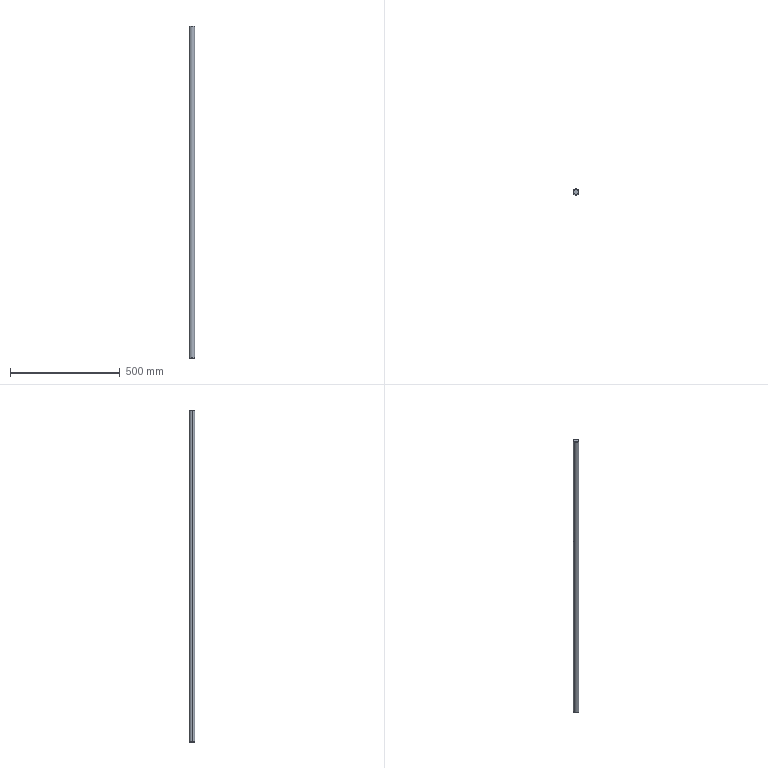Part | STEP file | 1 solid | 8 faces | box 25 x 25 x 1510 mm | volume 741143 mm3 | cone 4 | cylinder 2 | plane 2 | commonest cylinder face diameters 25 x2
STEP:
#1=CARTESIAN_POINT('',(0.,0.,0.));
#2=DIRECTION('',(0.,0.,1.));
#3=DIRECTION('',(1.,0.,0.));
#4=AXIS2_PLACEMENT_3D('',#1,#2,#3);
#5=CARTESIAN_POINT('',(-11.5,0.,-755.));
#6=VERTEX_POINT('',#5);
#7=CARTESIAN_POINT('',(11.5,0.,-755.));
#8=VERTEX_POINT('',#7);
#9=CARTESIAN_POINT('',(0.,0.,-755.));
#10=DIRECTION('',(0.,0.,-1.));
#11=DIRECTION('',(1.,0.,0.));
#12=AXIS2_PLACEMENT_3D('',#9,#10,#11);
#13=CIRCLE('',#12,11.5);
#14=CARTESIAN_POINT('',(0.,0.,-754.));
#15=DIRECTION('',(0.,0.,1.));
#16=DIRECTION('',(1.,0.,0.));
#17=AXIS2_PLACEMENT_3D('',#14,#15,#16);
#18=CONICAL_SURFACE('',#17,12.5,0.7854);
#19=CARTESIAN_POINT('',(6.283,-1.));
#20=DIRECTION('',(-1.,0.));
#21=VECTOR('',#20,1.);
#22=LINE('',#19,#21);
#23=(GEOMETRIC_REPRESENTATION_CONTEXT(2)PARAMETRIC_REPRESENTATION_CONTEXT()REPRESENTATION_CONTEXT('',''));
#24=DEFINITIONAL_REPRESENTATION('',(#22),#23);
#25=PCURVE('',#18,#24);
#26=CARTESIAN_POINT('',(0.,0.,-755.));
#27=DIRECTION('',(0.,0.,1.));
#28=DIRECTION('',(1.,0.,0.));
#29=AXIS2_PLACEMENT_3D('',#26,#27,#28);
#30=PLANE('',#29);
#31=CARTESIAN_POINT('',(11.5,0.));
#32=CARTESIAN_POINT('',(11.5,-19.919));
#33=CARTESIAN_POINT('',(-5.75,-9.959));
#34=CARTESIAN_POINT('',(-23.,0.));
#35=CARTESIAN_POINT('',(-5.75,9.959));
#36=CARTESIAN_POINT('',(11.5,19.919));
#37=CARTESIAN_POINT('',(11.5,0.));
#38=(BOUNDED_CURVE()B_SPLINE_CURVE(2,(#31,#32,#33,#34,#35,#36,#37),.UNSPECIFIED.,.T.,.F.)B_SPLINE_CURVE_WITH_KNOTS((1,2,2,2,2,1),(-2.094,0.,2.094,4.189,6.283,8.378),.UNSPECIFIED.)CURVE()GEOMETRIC_REPRESENTATION_ITEM()RATIONAL_B_SPLINE_CURVE((1.,0.5,1.,0.5,1.,0.5,1.))REPRESENTATION_ITEM(''));
#39=(GEOMETRIC_REPRESENTATION_CONTEXT(2)PARAMETRIC_REPRESENTATION_CONTEXT()REPRESENTATION_CONTEXT('',''));
#40=DEFINITIONAL_REPRESENTATION('',(#38),#39);
#41=PCURVE('',#30,#40);
#42=SURFACE_CURVE('',#13,(#25,#41),.PCURVE_S1.);
#43=EDGE_CURVE('',#6,#8,#42,.T.);
#44=ORIENTED_EDGE('',*,*,#43,.F.);
#45=CARTESIAN_POINT('',(-12.5,0.,-754.));
#46=VERTEX_POINT('',#45);
#47=CARTESIAN_POINT('',(-12.5,0.,-754.));
#48=DIRECTION('',(-0.7071,0.,0.7071));
#49=VECTOR('',#48,1.);
#50=LINE('',#47,#49);
#51=CARTESIAN_POINT('',(3.142,0.));
#52=DIRECTION('',(0.,1.));
#53=VECTOR('',#52,1.);
#54=LINE('',#51,#53);
#55=(GEOMETRIC_REPRESENTATION_CONTEXT(2)PARAMETRIC_REPRESENTATION_CONTEXT()REPRESENTATION_CONTEXT('',''));
#56=DEFINITIONAL_REPRESENTATION('',(#54),#55);
#57=PCURVE('',#18,#56);
#58=CARTESIAN_POINT('',(0.,0.,-754.));
#59=DIRECTION('',(0.,0.,1.));
#60=DIRECTION('',(1.,0.,0.));
#61=AXIS2_PLACEMENT_3D('',#58,#59,#60);
#62=CONICAL_SURFACE('',#61,12.5,0.7854);
#63=CARTESIAN_POINT('',(3.142,0.));
#64=DIRECTION('',(0.,1.));
#65=VECTOR('',#64,1.);
#66=LINE('',#63,#65);
#67=(GEOMETRIC_REPRESENTATION_CONTEXT(2)PARAMETRIC_REPRESENTATION_CONTEXT()REPRESENTATION_CONTEXT('',''));
#68=DEFINITIONAL_REPRESENTATION('',(#66),#67);
#69=PCURVE('',#62,#68);
#70=SURFACE_CURVE('',#50,(#57,#69),.PCURVE_S1.);
#71=EDGE_CURVE('',#6,#46,#70,.T.);
#72=ORIENTED_EDGE('',*,*,#71,.T.);
#73=CARTESIAN_POINT('',(12.5,0.,-754.));
#74=VERTEX_POINT('',#73);
#75=CARTESIAN_POINT('',(0.,0.,-754.));
#76=DIRECTION('',(0.,0.,1.));
#77=DIRECTION('',(1.,0.,0.));
#78=AXIS2_PLACEMENT_3D('',#75,#76,#77);
#79=CIRCLE('',#78,12.5);
#80=CARTESIAN_POINT('',(0.,0.));
#81=DIRECTION('',(1.,0.));
#82=VECTOR('',#81,1.);
#83=LINE('',#80,#82);
#84=(GEOMETRIC_REPRESENTATION_CONTEXT(2)PARAMETRIC_REPRESENTATION_CONTEXT()REPRESENTATION_CONTEXT('',''));
#85=DEFINITIONAL_REPRESENTATION('',(#83),#84);
#86=PCURVE('',#18,#85);
#87=CARTESIAN_POINT('',(0.,0.,755.));
#88=DIRECTION('',(0.,0.,-1.));
#89=DIRECTION('',(-1.,0.,0.));
#90=AXIS2_PLACEMENT_3D('',#87,#88,#89);
#91=CYLINDRICAL_SURFACE('',#90,12.5);
#92=CARTESIAN_POINT('',(3.142,1509.));
#93=DIRECTION('',(-1.,0.));
#94=VECTOR('',#93,1.);
#95=LINE('',#92,#94);
#96=(GEOMETRIC_REPRESENTATION_CONTEXT(2)PARAMETRIC_REPRESENTATION_CONTEXT()REPRESENTATION_CONTEXT('',''));
#97=DEFINITIONAL_REPRESENTATION('',(#95),#96);
#98=PCURVE('',#91,#97);
#99=SURFACE_CURVE('',#79,(#86,#98),.PCURVE_S1.);
#100=EDGE_CURVE('',#74,#46,#99,.T.);
#101=ORIENTED_EDGE('',*,*,#100,.F.);
#102=CARTESIAN_POINT('',(12.5,0.,-754.));
#103=DIRECTION('',(0.7071,0.,0.7071));
#104=VECTOR('',#103,1.);
#105=LINE('',#102,#104);
#106=CARTESIAN_POINT('',(0.,0.));
#107=DIRECTION('',(0.,1.));
#108=VECTOR('',#107,1.);
#109=LINE('',#106,#108);
#110=(GEOMETRIC_REPRESENTATION_CONTEXT(2)PARAMETRIC_REPRESENTATION_CONTEXT()REPRESENTATION_CONTEXT('',''));
#111=DEFINITIONAL_REPRESENTATION('',(#109),#110);
#112=PCURVE('',#18,#111);
#113=CARTESIAN_POINT('',(6.283,0.));
#114=DIRECTION('',(0.,1.));
#115=VECTOR('',#114,1.);
#116=LINE('',#113,#115);
#117=(GEOMETRIC_REPRESENTATION_CONTEXT(2)PARAMETRIC_REPRESENTATION_CONTEXT()REPRESENTATION_CONTEXT('',''));
#118=DEFINITIONAL_REPRESENTATION('',(#116),#117);
#119=PCURVE('',#62,#118);
#120=SURFACE_CURVE('',#105,(#112,#119),.PCURVE_S1.);
#121=EDGE_CURVE('',#8,#74,#120,.T.);
#122=ORIENTED_EDGE('',*,*,#121,.F.);
#123=EDGE_LOOP('',(#44,#72,#101,#122));
#124=FACE_BOUND('',#123,.T.);
#125=ADVANCED_FACE('',(#124),#18,.T.);
#126=CARTESIAN_POINT('',(11.5,0.,755.));
#127=VERTEX_POINT('',#126);
#128=CARTESIAN_POINT('',(-11.5,0.,755.));
#129=VERTEX_POINT('',#128);
#130=CARTESIAN_POINT('',(0.,0.,755.));
#131=DIRECTION('',(0.,0.,1.));
#132=DIRECTION('',(1.,0.,0.));
#133=AXIS2_PLACEMENT_3D('',#130,#131,#132);
#134=CIRCLE('',#133,11.5);
#135=CARTESIAN_POINT('',(0.,0.,755.));
#136=DIRECTION('',(0.,0.,-1.));
#137=DIRECTION('',(-1.,0.,0.));
#138=AXIS2_PLACEMENT_3D('',#135,#136,#137);
#139=CONICAL_SURFACE('',#138,11.5,0.7854);
#140=CARTESIAN_POINT('',(3.142,0.));
#141=DIRECTION('',(-1.,0.));
#142=VECTOR('',#141,1.);
#143=LINE('',#140,#142);
#144=(GEOMETRIC_REPRESENTATION_CONTEXT(2)PARAMETRIC_REPRESENTATION_CONTEXT()REPRESENTATION_CONTEXT('',''));
#145=DEFINITIONAL_REPRESENTATION('',(#143),#144);
#146=PCURVE('',#139,#145);
#147=CARTESIAN_POINT('',(0.,0.,755.));
#148=DIRECTION('',(0.,0.,1.));
#149=DIRECTION('',(1.,0.,0.));
#150=AXIS2_PLACEMENT_3D('',#147,#148,#149);
#151=PLANE('',#150);
#152=CARTESIAN_POINT('',(0.,0.));
#153=DIRECTION('',(1.,0.));
#154=AXIS2_PLACEMENT_2D('',#152,#153);
#155=CIRCLE('',#154,11.5);
#156=(GEOMETRIC_REPRESENTATION_CONTEXT(2)PARAMETRIC_REPRESENTATION_CONTEXT()REPRESENTATION_CONTEXT('',''));
#157=DEFINITIONAL_REPRESENTATION('',(#155),#156);
#158=PCURVE('',#151,#157);
#159=SURFACE_CURVE('',#134,(#146,#158),.PCURVE_S1.);
#160=EDGE_CURVE('',#127,#129,#159,.T.);
#161=ORIENTED_EDGE('',*,*,#160,.F.);
#162=CARTESIAN_POINT('',(12.5,0.,754.));
#163=VERTEX_POINT('',#162);
#164=CARTESIAN_POINT('',(11.5,0.,755.));
#165=DIRECTION('',(0.7071,0.,-0.7071));
#166=VECTOR('',#165,1.);
#167=LINE('',#164,#166);
#168=CARTESIAN_POINT('',(3.142,0.));
#169=DIRECTION('',(0.,1.));
#170=VECTOR('',#169,1.);
#171=LINE('',#168,#170);
#172=(GEOMETRIC_REPRESENTATION_CONTEXT(2)PARAMETRIC_REPRESENTATION_CONTEXT()REPRESENTATION_CONTEXT('',''));
#173=DEFINITIONAL_REPRESENTATION('',(#171),#172);
#174=PCURVE('',#139,#173);
#175=CARTESIAN_POINT('',(0.,0.,755.));
#176=DIRECTION('',(0.,0.,-1.));
#177=DIRECTION('',(-1.,0.,0.));
#178=AXIS2_PLACEMENT_3D('',#175,#176,#177);
#179=CONICAL_SURFACE('',#178,11.5,0.7854);
#180=CARTESIAN_POINT('',(3.142,0.));
#181=DIRECTION('',(0.,1.));
#182=VECTOR('',#181,1.);
#183=LINE('',#180,#182);
#184=(GEOMETRIC_REPRESENTATION_CONTEXT(2)PARAMETRIC_REPRESENTATION_CONTEXT()REPRESENTATION_CONTEXT('',''));
#185=DEFINITIONAL_REPRESENTATION('',(#183),#184);
#186=PCURVE('',#179,#185);
#187=SURFACE_CURVE('',#167,(#174,#186),.PCURVE_S1.);
#188=EDGE_CURVE('',#127,#163,#187,.T.);
#189=ORIENTED_EDGE('',*,*,#188,.T.);
#190=CARTESIAN_POINT('',(-12.5,0.,754.));
#191=VERTEX_POINT('',#190);
#192=CARTESIAN_POINT('',(0.,0.,754.));
#193=DIRECTION('',(0.,0.,-1.));
#194=DIRECTION('',(1.,0.,0.));
#195=AXIS2_PLACEMENT_3D('',#192,#193,#194);
#196=CIRCLE('',#195,12.5);
#197=CARTESIAN_POINT('',(-3.142,1.));
#198=DIRECTION('',(1.,0.));
#199=VECTOR('',#198,1.);
#200=LINE('',#197,#199);
#201=(GEOMETRIC_REPRESENTATION_CONTEXT(2)PARAMETRIC_REPRESENTATION_CONTEXT()REPRESENTATION_CONTEXT('',''));
#202=DEFINITIONAL_REPRESENTATION('',(#200),#201);
#203=PCURVE('',#139,#202);
#204=CARTESIAN_POINT('',(-3.142,1.));
#205=DIRECTION('',(1.,0.));
#206=VECTOR('',#205,1.);
#207=LINE('',#204,#206);
#208=(GEOMETRIC_REPRESENTATION_CONTEXT(2)PARAMETRIC_REPRESENTATION_CONTEXT()REPRESENTATION_CONTEXT('',''));
#209=DEFINITIONAL_REPRESENTATION('',(#207),#208);
#210=PCURVE('',#91,#209);
#211=SURFACE_CURVE('',#196,(#203,#210),.PCURVE_S1.);
#212=EDGE_CURVE('',#191,#163,#211,.T.);
#213=ORIENTED_EDGE('',*,*,#212,.F.);
#214=CARTESIAN_POINT('',(-11.5,0.,755.));
#215=DIRECTION('',(-0.7071,0.,-0.7071));
#216=VECTOR('',#215,1.);
#217=LINE('',#214,#216);
#218=CARTESIAN_POINT('',(0.,0.));
#219=DIRECTION('',(0.,1.));
#220=VECTOR('',#219,1.);
#221=LINE('',#218,#220);
#222=(GEOMETRIC_REPRESENTATION_CONTEXT(2)PARAMETRIC_REPRESENTATION_CONTEXT()REPRESENTATION_CONTEXT('',''));
#223=DEFINITIONAL_REPRESENTATION('',(#221),#222);
#224=PCURVE('',#139,#223);
#225=CARTESIAN_POINT('',(6.283,0.));
#226=DIRECTION('',(0.,1.));
#227=VECTOR('',#226,1.);
#228=LINE('',#225,#227);
#229=(GEOMETRIC_REPRESENTATION_CONTEXT(2)PARAMETRIC_REPRESENTATION_CONTEXT()REPRESENTATION_CONTEXT('',''));
#230=DEFINITIONAL_REPRESENTATION('',(#228),#229);
#231=PCURVE('',#179,#230);
#232=SURFACE_CURVE('',#217,(#224,#231),.PCURVE_S1.);
#233=EDGE_CURVE('',#129,#191,#232,.T.);
#234=ORIENTED_EDGE('',*,*,#233,.F.);
#235=EDGE_LOOP('',(#161,#189,#213,#234));
#236=FACE_BOUND('',#235,.T.);
#237=ADVANCED_FACE('',(#236),#139,.T.);
#238=ORIENTED_EDGE('',*,*,#212,.T.);
#239=CARTESIAN_POINT('',(12.5,0.,755.));
#240=DIRECTION('',(0.,0.,-1.));
#241=VECTOR('',#240,1.);
#242=LINE('',#239,#241);
#243=CARTESIAN_POINT('',(3.142,0.));
#244=DIRECTION('',(0.,1.));
#245=VECTOR('',#244,1.);
#246=LINE('',#243,#245);
#247=(GEOMETRIC_REPRESENTATION_CONTEXT(2)PARAMETRIC_REPRESENTATION_CONTEXT()REPRESENTATION_CONTEXT('',''));
#248=DEFINITIONAL_REPRESENTATION('',(#246),#247);
#249=PCURVE('',#91,#248);
#250=CARTESIAN_POINT('',(0.,0.,755.));
#251=DIRECTION('',(0.,0.,-1.));
#252=DIRECTION('',(-1.,0.,0.));
#253=AXIS2_PLACEMENT_3D('',#250,#251,#252);
#254=CYLINDRICAL_SURFACE('',#253,12.5);
#255=CARTESIAN_POINT('',(3.142,0.));
#256=DIRECTION('',(0.,1.));
#257=VECTOR('',#256,1.);
#258=LINE('',#255,#257);
#259=(GEOMETRIC_REPRESENTATION_CONTEXT(2)PARAMETRIC_REPRESENTATION_CONTEXT()REPRESENTATION_CONTEXT('',''));
#260=DEFINITIONAL_REPRESENTATION('',(#258),#259);
#261=PCURVE('',#254,#260);
#262=SURFACE_CURVE('',#242,(#249,#261),.PCURVE_S1.);
#263=EDGE_CURVE('',#163,#74,#262,.T.);
#264=ORIENTED_EDGE('',*,*,#263,.T.);
#265=ORIENTED_EDGE('',*,*,#100,.T.);
#266=CARTESIAN_POINT('',(-12.5,0.,755.));
#267=DIRECTION('',(0.,0.,-1.));
#268=VECTOR('',#267,1.);
#269=LINE('',#266,#268);
#270=CARTESIAN_POINT('',(0.,0.));
#271=DIRECTION('',(0.,1.));
#272=VECTOR('',#271,1.);
#273=LINE('',#270,#272);
#274=(GEOMETRIC_REPRESENTATION_CONTEXT(2)PARAMETRIC_REPRESENTATION_CONTEXT()REPRESENTATION_CONTEXT('',''));
#275=DEFINITIONAL_REPRESENTATION('',(#273),#274);
#276=PCURVE('',#91,#275);
#277=CARTESIAN_POINT('',(6.283,0.));
#278=DIRECTION('',(0.,1.));
#279=VECTOR('',#278,1.);
#280=LINE('',#277,#279);
#281=(GEOMETRIC_REPRESENTATION_CONTEXT(2)PARAMETRIC_REPRESENTATION_CONTEXT()REPRESENTATION_CONTEXT('',''));
#282=DEFINITIONAL_REPRESENTATION('',(#280),#281);
#283=PCURVE('',#254,#282);
#284=SURFACE_CURVE('',#269,(#276,#283),.PCURVE_S1.);
#285=EDGE_CURVE('',#191,#46,#284,.T.);
#286=ORIENTED_EDGE('',*,*,#285,.F.);
#287=EDGE_LOOP('',(#238,#264,#265,#286));
#288=FACE_BOUND('',#287,.T.);
#289=ADVANCED_FACE('',(#288),#91,.T.);
#290=ORIENTED_EDGE('',*,*,#263,.F.);
#291=CARTESIAN_POINT('',(0.,0.,754.));
#292=DIRECTION('',(0.,0.,-1.));
#293=DIRECTION('',(1.,0.,0.));
#294=AXIS2_PLACEMENT_3D('',#291,#292,#293);
#295=CIRCLE('',#294,12.5);
#296=CARTESIAN_POINT('',(3.142,1.));
#297=DIRECTION('',(1.,0.));
#298=VECTOR('',#297,1.);
#299=LINE('',#296,#298);
#300=(GEOMETRIC_REPRESENTATION_CONTEXT(2)PARAMETRIC_REPRESENTATION_CONTEXT()REPRESENTATION_CONTEXT('',''));
#301=DEFINITIONAL_REPRESENTATION('',(#299),#300);
#302=PCURVE('',#254,#301);
#303=CARTESIAN_POINT('',(3.142,1.));
#304=DIRECTION('',(1.,0.));
#305=VECTOR('',#304,1.);
#306=LINE('',#303,#305);
#307=(GEOMETRIC_REPRESENTATION_CONTEXT(2)PARAMETRIC_REPRESENTATION_CONTEXT()REPRESENTATION_CONTEXT('',''));
#308=DEFINITIONAL_REPRESENTATION('',(#306),#307);
#309=PCURVE('',#179,#308);
#310=SURFACE_CURVE('',#295,(#302,#309),.PCURVE_S1.);
#311=EDGE_CURVE('',#163,#191,#310,.T.);
#312=ORIENTED_EDGE('',*,*,#311,.T.);
#313=ORIENTED_EDGE('',*,*,#285,.T.);
#314=CARTESIAN_POINT('',(0.,0.,-754.));
#315=DIRECTION('',(0.,0.,1.));
#316=DIRECTION('',(1.,0.,0.));
#317=AXIS2_PLACEMENT_3D('',#314,#315,#316);
#318=CIRCLE('',#317,12.5);
#319=CARTESIAN_POINT('',(9.425,1509.));
#320=DIRECTION('',(-1.,0.));
#321=VECTOR('',#320,1.);
#322=LINE('',#319,#321);
#323=(GEOMETRIC_REPRESENTATION_CONTEXT(2)PARAMETRIC_REPRESENTATION_CONTEXT()REPRESENTATION_CONTEXT('',''));
#324=DEFINITIONAL_REPRESENTATION('',(#322),#323);
#325=PCURVE('',#254,#324);
#326=CARTESIAN_POINT('',(0.,0.));
#327=DIRECTION('',(1.,0.));
#328=VECTOR('',#327,1.);
#329=LINE('',#326,#328);
#330=(GEOMETRIC_REPRESENTATION_CONTEXT(2)PARAMETRIC_REPRESENTATION_CONTEXT()REPRESENTATION_CONTEXT('',''));
#331=DEFINITIONAL_REPRESENTATION('',(#329),#330);
#332=PCURVE('',#62,#331);
#333=SURFACE_CURVE('',#318,(#325,#332),.PCURVE_S1.);
#334=EDGE_CURVE('',#46,#74,#333,.T.);
#335=ORIENTED_EDGE('',*,*,#334,.T.);
#336=EDGE_LOOP('',(#290,#312,#313,#335));
#337=FACE_BOUND('',#336,.T.);
#338=ADVANCED_FACE('',(#337),#254,.T.);
#339=CARTESIAN_POINT('',(0.,0.,755.));
#340=DIRECTION('',(0.,0.,1.));
#341=DIRECTION('',(1.,0.,0.));
#342=AXIS2_PLACEMENT_3D('',#339,#340,#341);
#343=CIRCLE('',#342,11.5);
#344=CARTESIAN_POINT('',(0.,0.));
#345=DIRECTION('',(1.,0.));
#346=AXIS2_PLACEMENT_2D('',#344,#345);
#347=CIRCLE('',#346,11.5);
#348=(GEOMETRIC_REPRESENTATION_CONTEXT(2)PARAMETRIC_REPRESENTATION_CONTEXT()REPRESENTATION_CONTEXT('',''));
#349=DEFINITIONAL_REPRESENTATION('',(#347),#348);
#350=PCURVE('',#151,#349);
#351=CARTESIAN_POINT('',(9.425,0.));
#352=DIRECTION('',(-1.,0.));
#353=VECTOR('',#352,1.);
#354=LINE('',#351,#353);
#355=(GEOMETRIC_REPRESENTATION_CONTEXT(2)PARAMETRIC_REPRESENTATION_CONTEXT()REPRESENTATION_CONTEXT('',''));
#356=DEFINITIONAL_REPRESENTATION('',(#354),#355);
#357=PCURVE('',#179,#356);
#358=SURFACE_CURVE('',#343,(#350,#357),.PCURVE_S1.);
#359=EDGE_CURVE('',#129,#127,#358,.T.);
#360=ORIENTED_EDGE('',*,*,#359,.T.);
#361=ORIENTED_EDGE('',*,*,#160,.T.);
#362=EDGE_LOOP('',(#360,#361));
#363=FACE_BOUND('',#362,.T.);
#364=ADVANCED_FACE('',(#363),#151,.T.);
#365=CARTESIAN_POINT('',(0.,0.,-755.));
#366=DIRECTION('',(0.,0.,-1.));
#367=DIRECTION('',(1.,0.,0.));
#368=AXIS2_PLACEMENT_3D('',#365,#366,#367);
#369=CIRCLE('',#368,11.5);
#370=CARTESIAN_POINT('',(11.5,0.));
#371=CARTESIAN_POINT('',(11.5,-19.919));
#372=CARTESIAN_POINT('',(-5.75,-9.959));
#373=CARTESIAN_POINT('',(-23.,0.));
#374=CARTESIAN_POINT('',(-5.75,9.959));
#375=CARTESIAN_POINT('',(11.5,19.919));
#376=CARTESIAN_POINT('',(11.5,0.));
#377=(BOUNDED_CURVE()B_SPLINE_CURVE(2,(#370,#371,#372,#373,#374,#375,#376),.UNSPECIFIED.,.T.,.F.)B_SPLINE_CURVE_WITH_KNOTS((1,2,2,2,2,1),(-2.094,0.,2.094,4.189,6.283,8.378),.UNSPECIFIED.)CURVE()GEOMETRIC_REPRESENTATION_ITEM()RATIONAL_B_SPLINE_CURVE((1.,0.5,1.,0.5,1.,0.5,1.))REPRESENTATION_ITEM(''));
#378=(GEOMETRIC_REPRESENTATION_CONTEXT(2)PARAMETRIC_REPRESENTATION_CONTEXT()REPRESENTATION_CONTEXT('',''));
#379=DEFINITIONAL_REPRESENTATION('',(#377),#378);
#380=PCURVE('',#30,#379);
#381=CARTESIAN_POINT('',(6.283,-1.));
#382=DIRECTION('',(-1.,0.));
#383=VECTOR('',#382,1.);
#384=LINE('',#381,#383);
#385=(GEOMETRIC_REPRESENTATION_CONTEXT(2)PARAMETRIC_REPRESENTATION_CONTEXT()REPRESENTATION_CONTEXT('',''));
#386=DEFINITIONAL_REPRESENTATION('',(#384),#385);
#387=PCURVE('',#62,#386);
#388=SURFACE_CURVE('',#369,(#380,#387),.PCURVE_S1.);
#389=EDGE_CURVE('',#8,#6,#388,.T.);
#390=ORIENTED_EDGE('',*,*,#389,.T.);
#391=ORIENTED_EDGE('',*,*,#43,.T.);
#392=EDGE_LOOP('',(#390,#391));
#393=FACE_BOUND('',#392,.T.);
#394=ADVANCED_FACE('',(#393),#30,.F.);
#395=ORIENTED_EDGE('',*,*,#188,.F.);
#396=ORIENTED_EDGE('',*,*,#359,.F.);
#397=ORIENTED_EDGE('',*,*,#233,.T.);
#398=ORIENTED_EDGE('',*,*,#311,.F.);
#399=EDGE_LOOP('',(#395,#396,#397,#398));
#400=FACE_BOUND('',#399,.T.);
#401=ADVANCED_FACE('',(#400),#179,.T.);
#402=ORIENTED_EDGE('',*,*,#71,.F.);
#403=ORIENTED_EDGE('',*,*,#389,.F.);
#404=ORIENTED_EDGE('',*,*,#121,.T.);
#405=ORIENTED_EDGE('',*,*,#334,.F.);
#406=EDGE_LOOP('',(#402,#403,#404,#405));
#407=FACE_BOUND('',#406,.T.);
#408=ADVANCED_FACE('',(#407),#62,.T.);
#409=CLOSED_SHELL('',(#125,#237,#289,#338,#364,#394,#401,#408));
#410=MANIFOLD_SOLID_BREP('',#409);
#411=(LENGTH_UNIT()NAMED_UNIT(*)SI_UNIT(.MILLI.,.METRE.));
#412=UNCERTAINTY_MEASURE_WITH_UNIT(LENGTH_MEASURE(0.0000001),#411,'','');
#413=(NAMED_UNIT(*)PLANE_ANGLE_UNIT()SI_UNIT($,.RADIAN.));
#414=(NAMED_UNIT(*)SI_UNIT($,.STERADIAN.)SOLID_ANGLE_UNIT());
#415=(GEOMETRIC_REPRESENTATION_CONTEXT(3)GLOBAL_UNCERTAINTY_ASSIGNED_CONTEXT((#412))GLOBAL_UNIT_ASSIGNED_CONTEXT((#411,#413,#414))REPRESENTATION_CONTEXT('',''));
#416=ADVANCED_BREP_SHAPE_REPRESENTATION('',(#4,#410),#415);